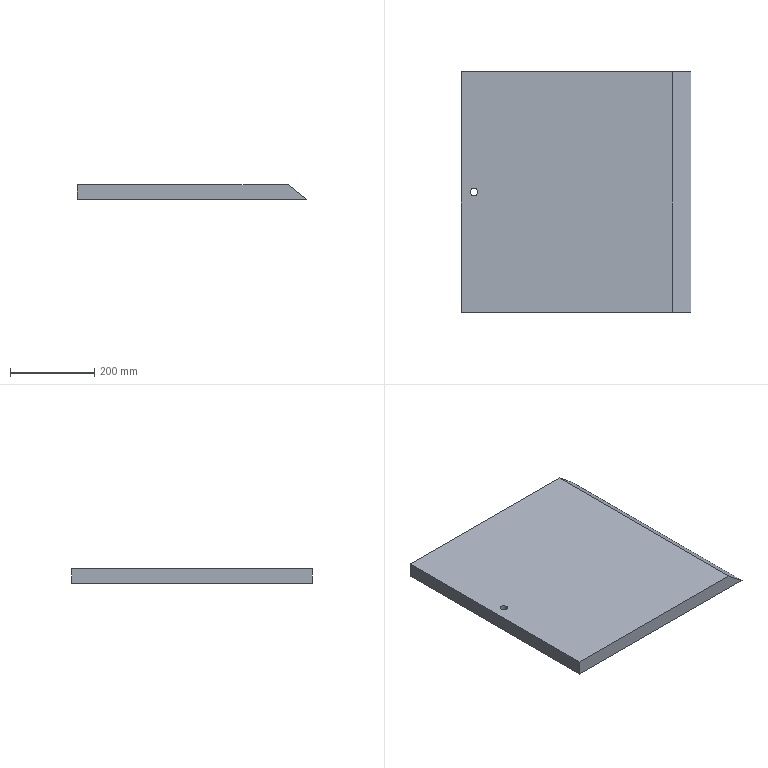Part | SolidWorks | features 3DProfileFeature 1, Cut 1, Extrusion 1, HoleWzd 1 | 1 solid | 8 faces | box 543.75 x 570 x 35 mm | volume 10402988 mm3 | plane 6 | cylinder 2 | commonest cylinder face diameters 17.5 x2
STEP:
#1=CARTESIAN_POINT('',(21.25,285.,0.));
#2=VERTEX_POINT('',#1);
#3=CARTESIAN_POINT('',(38.75,285.,0.));
#4=VERTEX_POINT('',#3);
#5=CARTESIAN_POINT('',(30.,285.,0.));
#6=DIRECTION('',(0.,0.,1.));
#7=DIRECTION('',(1.,0.,0.));
#8=AXIS2_PLACEMENT_3D('',#5,#6,#7);
#9=CIRCLE('',#8,8.75);
#10=EDGE_CURVE('',#2,#4,#9,.T.);
#11=ORIENTED_EDGE('',*,*,#10,.F.);
#12=CARTESIAN_POINT('',(21.25,285.,35.));
#13=VERTEX_POINT('',#12);
#14=CARTESIAN_POINT('',(21.25,285.,35.));
#15=DIRECTION('',(0.,0.,1.));
#16=VECTOR('',#15,1000.);
#17=LINE('',#14,#16);
#18=EDGE_CURVE('',#2,#13,#17,.T.);
#19=ORIENTED_EDGE('',*,*,#18,.T.);
#20=CARTESIAN_POINT('',(38.75,285.,35.));
#21=VERTEX_POINT('',#20);
#22=CARTESIAN_POINT('',(30.,285.,35.));
#23=DIRECTION('',(0.,0.,1.));
#24=DIRECTION('',(1.,0.,0.));
#25=AXIS2_PLACEMENT_3D('',#22,#23,#24);
#26=CIRCLE('',#25,8.75);
#27=EDGE_CURVE('',#13,#21,#26,.T.);
#28=ORIENTED_EDGE('',*,*,#27,.T.);
#29=CARTESIAN_POINT('',(38.75,285.,35.));
#30=DIRECTION('',(0.,0.,1.));
#31=VECTOR('',#30,1000.);
#32=LINE('',#29,#31);
#33=EDGE_CURVE('',#4,#21,#32,.T.);
#34=ORIENTED_EDGE('',*,*,#33,.F.);
#35=EDGE_LOOP('',(#11,#19,#28,#34));
#36=FACE_OUTER_BOUND('',#35,.T.);
#37=CARTESIAN_POINT('',(30.,285.,35.));
#38=DIRECTION('',(0.,0.,1.));
#39=DIRECTION('',(1.,0.,0.));
#40=AXIS2_PLACEMENT_3D('',#37,#38,#39);
#41=CYLINDRICAL_SURFACE('',#40,8.75);
#42=ADVANCED_FACE('',(#36),#41,.F.);
#43=CARTESIAN_POINT('',(500.,570.,35.));
#44=VERTEX_POINT('',#43);
#45=CARTESIAN_POINT('',(543.75,570.,0.));
#46=VERTEX_POINT('',#45);
#47=CARTESIAN_POINT('',(1000.,570.,-365.));
#48=DIRECTION('',(0.7809,0.,-0.6247));
#49=VECTOR('',#48,1000.);
#50=LINE('',#47,#49);
#51=EDGE_CURVE('',#44,#46,#50,.T.);
#52=ORIENTED_EDGE('',*,*,#51,.T.);
#53=CARTESIAN_POINT('',(0.,570.,0.));
#54=VERTEX_POINT('',#53);
#55=CARTESIAN_POINT('',(0.,570.,0.));
#56=DIRECTION('',(1.,0.,0.));
#57=VECTOR('',#56,1000.);
#58=LINE('',#55,#57);
#59=EDGE_CURVE('',#54,#46,#58,.T.);
#60=ORIENTED_EDGE('',*,*,#59,.F.);
#61=CARTESIAN_POINT('',(0.,570.,35.));
#62=VERTEX_POINT('',#61);
#63=CARTESIAN_POINT('',(0.,570.,35.));
#64=DIRECTION('',(0.,0.,-1.));
#65=VECTOR('',#64,1000.);
#66=LINE('',#63,#65);
#67=EDGE_CURVE('',#62,#54,#66,.T.);
#68=ORIENTED_EDGE('',*,*,#67,.F.);
#69=CARTESIAN_POINT('',(0.,570.,35.));
#70=DIRECTION('',(1.,0.,0.));
#71=VECTOR('',#70,1000.);
#72=LINE('',#69,#71);
#73=EDGE_CURVE('',#62,#44,#72,.T.);
#74=ORIENTED_EDGE('',*,*,#73,.T.);
#75=EDGE_LOOP('',(#52,#60,#68,#74));
#76=FACE_OUTER_BOUND('',#75,.T.);
#77=CARTESIAN_POINT('',(0.,570.,35.));
#78=DIRECTION('',(0.,1.,0.));
#79=DIRECTION('',(0.,0.,1.));
#80=AXIS2_PLACEMENT_3D('',#77,#78,#79);
#81=PLANE('',#80);
#82=ADVANCED_FACE('',(#76),#81,.T.);
#83=CARTESIAN_POINT('',(0.,0.,0.));
#84=VERTEX_POINT('',#83);
#85=CARTESIAN_POINT('',(0.,570.,0.));
#86=DIRECTION('',(0.,-1.,0.));
#87=VECTOR('',#86,1000.);
#88=LINE('',#85,#87);
#89=EDGE_CURVE('',#54,#84,#88,.T.);
#90=ORIENTED_EDGE('',*,*,#89,.T.);
#91=CARTESIAN_POINT('',(0.,0.,35.));
#92=VERTEX_POINT('',#91);
#93=CARTESIAN_POINT('',(0.,0.,35.));
#94=DIRECTION('',(0.,0.,-1.));
#95=VECTOR('',#94,1000.);
#96=LINE('',#93,#95);
#97=EDGE_CURVE('',#92,#84,#96,.T.);
#98=ORIENTED_EDGE('',*,*,#97,.F.);
#99=CARTESIAN_POINT('',(0.,570.,35.));
#100=DIRECTION('',(0.,-1.,0.));
#101=VECTOR('',#100,1000.);
#102=LINE('',#99,#101);
#103=EDGE_CURVE('',#62,#92,#102,.T.);
#104=ORIENTED_EDGE('',*,*,#103,.F.);
#105=ORIENTED_EDGE('',*,*,#67,.T.);
#106=EDGE_LOOP('',(#90,#98,#104,#105));
#107=FACE_OUTER_BOUND('',#106,.T.);
#108=CARTESIAN_POINT('',(0.,570.,35.));
#109=DIRECTION('',(1.,0.,0.));
#110=DIRECTION('',(0.,1.,0.));
#111=AXIS2_PLACEMENT_3D('',#108,#109,#110);
#112=PLANE('',#111);
#113=ADVANCED_FACE('',(#107),#112,.F.);
#114=CARTESIAN_POINT('',(543.75,0.,0.));
#115=VERTEX_POINT('',#114);
#116=CARTESIAN_POINT('',(0.,0.,0.));
#117=DIRECTION('',(1.,0.,0.));
#118=VECTOR('',#117,1000.);
#119=LINE('',#116,#118);
#120=EDGE_CURVE('',#84,#115,#119,.T.);
#121=ORIENTED_EDGE('',*,*,#120,.T.);
#122=CARTESIAN_POINT('',(500.,0.,35.));
#123=VERTEX_POINT('',#122);
#124=CARTESIAN_POINT('',(1000.,0.,-365.));
#125=DIRECTION('',(0.7809,0.,-0.6247));
#126=VECTOR('',#125,1000.);
#127=LINE('',#124,#126);
#128=EDGE_CURVE('',#123,#115,#127,.T.);
#129=ORIENTED_EDGE('',*,*,#128,.F.);
#130=CARTESIAN_POINT('',(0.,0.,35.));
#131=DIRECTION('',(1.,0.,0.));
#132=VECTOR('',#131,1000.);
#133=LINE('',#130,#132);
#134=EDGE_CURVE('',#92,#123,#133,.T.);
#135=ORIENTED_EDGE('',*,*,#134,.F.);
#136=ORIENTED_EDGE('',*,*,#97,.T.);
#137=EDGE_LOOP('',(#121,#129,#135,#136));
#138=FACE_OUTER_BOUND('',#137,.T.);
#139=CARTESIAN_POINT('',(0.,0.,35.));
#140=DIRECTION('',(0.,1.,0.));
#141=DIRECTION('',(0.,0.,1.));
#142=AXIS2_PLACEMENT_3D('',#139,#140,#141);
#143=PLANE('',#142);
#144=ADVANCED_FACE('',(#138),#143,.F.);
#145=CARTESIAN_POINT('',(30.,285.,35.));
#146=DIRECTION('',(0.,0.,1.));
#147=DIRECTION('',(1.,0.,0.));
#148=AXIS2_PLACEMENT_3D('',#145,#146,#147);
#149=CIRCLE('',#148,8.75);
#150=EDGE_CURVE('',#21,#13,#149,.T.);
#151=ORIENTED_EDGE('',*,*,#150,.F.);
#152=ORIENTED_EDGE('',*,*,#27,.F.);
#153=EDGE_LOOP('',(#151,#152));
#154=FACE_BOUND('',#153,.T.);
#155=ORIENTED_EDGE('',*,*,#134,.T.);
#156=CARTESIAN_POINT('',(500.,570.,35.));
#157=DIRECTION('',(0.,-1.,0.));
#158=VECTOR('',#157,1000.);
#159=LINE('',#156,#158);
#160=EDGE_CURVE('',#44,#123,#159,.T.);
#161=ORIENTED_EDGE('',*,*,#160,.F.);
#162=ORIENTED_EDGE('',*,*,#73,.F.);
#163=ORIENTED_EDGE('',*,*,#103,.T.);
#164=EDGE_LOOP('',(#155,#161,#162,#163));
#165=FACE_OUTER_BOUND('',#164,.T.);
#166=CARTESIAN_POINT('',(0.,0.,35.));
#167=DIRECTION('',(0.,0.,-1.));
#168=DIRECTION('',(-1.,0.,0.));
#169=AXIS2_PLACEMENT_3D('',#166,#167,#168);
#170=PLANE('',#169);
#171=ADVANCED_FACE('',(#154,#165),#170,.F.);
#172=CARTESIAN_POINT('',(543.75,0.,0.));
#173=DIRECTION('',(0.,1.,0.));
#174=VECTOR('',#173,1000.);
#175=LINE('',#172,#174);
#176=EDGE_CURVE('',#115,#46,#175,.T.);
#177=ORIENTED_EDGE('',*,*,#176,.F.);
#178=ORIENTED_EDGE('',*,*,#120,.F.);
#179=ORIENTED_EDGE('',*,*,#89,.F.);
#180=ORIENTED_EDGE('',*,*,#59,.T.);
#181=EDGE_LOOP('',(#177,#178,#179,#180));
#182=FACE_OUTER_BOUND('',#181,.T.);
#183=CARTESIAN_POINT('',(30.,285.,0.));
#184=DIRECTION('',(0.,0.,1.));
#185=DIRECTION('',(1.,0.,0.));
#186=AXIS2_PLACEMENT_3D('',#183,#184,#185);
#187=CIRCLE('',#186,8.75);
#188=EDGE_CURVE('',#4,#2,#187,.T.);
#189=ORIENTED_EDGE('',*,*,#188,.T.);
#190=ORIENTED_EDGE('',*,*,#10,.T.);
#191=EDGE_LOOP('',(#189,#190));
#192=FACE_BOUND('',#191,.T.);
#193=CARTESIAN_POINT('',(0.,0.,0.));
#194=DIRECTION('',(0.,0.,-1.));
#195=DIRECTION('',(-1.,0.,0.));
#196=AXIS2_PLACEMENT_3D('',#193,#194,#195);
#197=PLANE('',#196);
#198=ADVANCED_FACE('',(#182,#192),#197,.T.);
#199=ORIENTED_EDGE('',*,*,#18,.F.);
#200=ORIENTED_EDGE('',*,*,#188,.F.);
#201=ORIENTED_EDGE('',*,*,#33,.T.);
#202=ORIENTED_EDGE('',*,*,#150,.T.);
#203=EDGE_LOOP('',(#199,#200,#201,#202));
#204=FACE_OUTER_BOUND('',#203,.T.);
#205=CARTESIAN_POINT('',(30.,285.,35.));
#206=DIRECTION('',(0.,0.,1.));
#207=DIRECTION('',(1.,0.,0.));
#208=AXIS2_PLACEMENT_3D('',#205,#206,#207);
#209=CYLINDRICAL_SURFACE('',#208,8.75);
#210=ADVANCED_FACE('',(#204),#209,.F.);
#211=ORIENTED_EDGE('',*,*,#176,.T.);
#212=ORIENTED_EDGE('',*,*,#51,.F.);
#213=ORIENTED_EDGE('',*,*,#160,.T.);
#214=ORIENTED_EDGE('',*,*,#128,.T.);
#215=EDGE_LOOP('',(#211,#212,#213,#214));
#216=FACE_OUTER_BOUND('',#215,.T.);
#217=CARTESIAN_POINT('',(1000.,570.,-365.));
#218=DIRECTION('',(-0.6247,0.,-0.7809));
#219=DIRECTION('',(-0.7809,0.,0.6247));
#220=AXIS2_PLACEMENT_3D('',#217,#218,#219);
#221=PLANE('',#220);
#222=ADVANCED_FACE('',(#216),#221,.F.);
#223=CLOSED_SHELL('',(#42,#82,#113,#144,#171,#198,#210,#222));
#224=MANIFOLD_SOLID_BREP('',#223);
#225=CARTESIAN_POINT('',(0.,0.,0.));
#226=DIRECTION('',(0.,0.,1.));
#227=DIRECTION('',(1.,0.,0.));
#228=AXIS2_PLACEMENT_3D('',#225,#226,#227);
#229=(LENGTH_UNIT()NAMED_UNIT(*)SI_UNIT(.MILLI.,.METRE.));
#230=UNCERTAINTY_MEASURE_WITH_UNIT(LENGTH_MEASURE(0.00001),#229,'','');
#231=(NAMED_UNIT(*)PLANE_ANGLE_UNIT()SI_UNIT($,.RADIAN.));
#232=(NAMED_UNIT(*)SI_UNIT($,.STERADIAN.)SOLID_ANGLE_UNIT());
#233=(GEOMETRIC_REPRESENTATION_CONTEXT(3)GLOBAL_UNCERTAINTY_ASSIGNED_CONTEXT((#230))GLOBAL_UNIT_ASSIGNED_CONTEXT((#229,#231,#232))REPRESENTATION_CONTEXT('',''));
#234=ADVANCED_BREP_SHAPE_REPRESENTATION('',(#224,#228),#233);